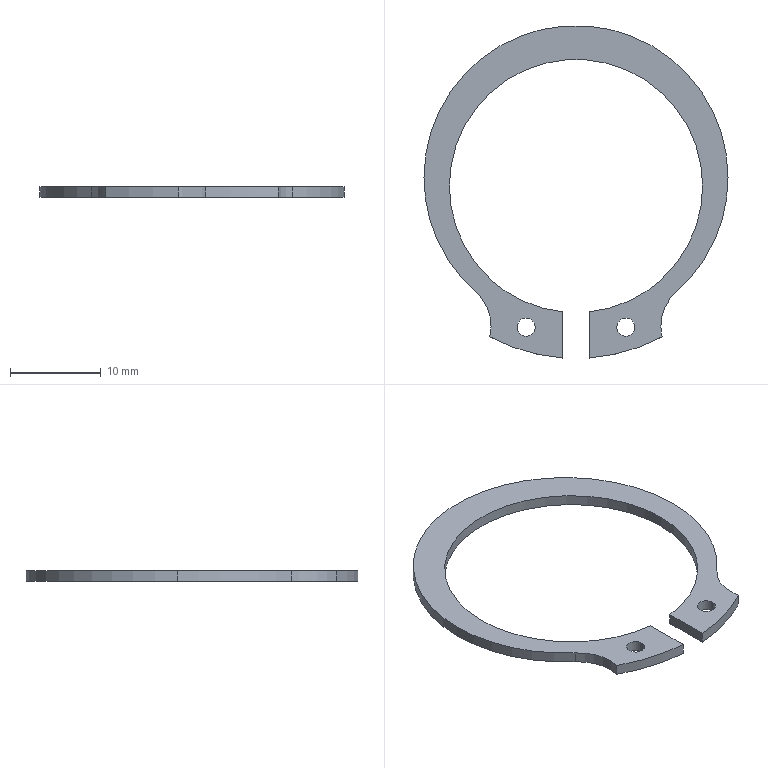Part | SolidWorks | features MBimport 1 | 1 solid | 19 faces | box 33.5 x 36.623 x 1.2 mm | volume 375.357 mm3 | cylinder 15 | plane 4 | commonest cylinder face diameters 2 x4 10 x3 27.9 x3 33.5 x3 39.86 x2
STEP:
#1=CARTESIAN_POINT('',(4.5,-16.486,0.6));
#2=VERTEX_POINT('',#1);
#3=CARTESIAN_POINT('',(6.5,-16.486,0.6));
#4=VERTEX_POINT('',#3);
#5=CARTESIAN_POINT('',(5.5,-16.486,0.6));
#6=DIRECTION('',(0.,0.,1.));
#7=DIRECTION('',(-1.,0.,0.));
#8=AXIS2_PLACEMENT_3D('',#5,#6,#7);
#9=CIRCLE('',#8,1.);
#10=EDGE_CURVE('',#2,#4,#9,.T.);
#11=ORIENTED_EDGE('',*,*,#10,.T.);
#12=CARTESIAN_POINT('',(6.5,-16.486,-0.6));
#13=VERTEX_POINT('',#12);
#14=CARTESIAN_POINT('',(6.5,-16.486,0.6));
#15=DIRECTION('',(0.,0.,-1.));
#16=VECTOR('',#15,1000.);
#17=LINE('',#14,#16);
#18=EDGE_CURVE('',#4,#13,#17,.T.);
#19=ORIENTED_EDGE('',*,*,#18,.T.);
#20=CARTESIAN_POINT('',(4.5,-16.486,-0.6));
#21=VERTEX_POINT('',#20);
#22=CARTESIAN_POINT('',(5.5,-16.486,-0.6));
#23=DIRECTION('',(0.,0.,1.));
#24=DIRECTION('',(-1.,0.,0.));
#25=AXIS2_PLACEMENT_3D('',#22,#23,#24);
#26=CIRCLE('',#25,1.);
#27=EDGE_CURVE('',#21,#13,#26,.T.);
#28=ORIENTED_EDGE('',*,*,#27,.F.);
#29=CARTESIAN_POINT('',(4.5,-16.486,0.6));
#30=DIRECTION('',(0.,0.,-1.));
#31=VECTOR('',#30,1000.);
#32=LINE('',#29,#31);
#33=EDGE_CURVE('',#2,#21,#32,.T.);
#34=ORIENTED_EDGE('',*,*,#33,.F.);
#35=EDGE_LOOP('',(#11,#19,#28,#34));
#36=FACE_OUTER_BOUND('',#35,.T.);
#37=CARTESIAN_POINT('',(5.5,-16.486,0.6));
#38=DIRECTION('',(0.,0.,-1.));
#39=DIRECTION('',(-1.,0.,0.));
#40=AXIS2_PLACEMENT_3D('',#37,#38,#39);
#41=CYLINDRICAL_SURFACE('',#40,1.);
#42=ADVANCED_FACE('',(#36),#41,.F.);
#43=CARTESIAN_POINT('',(-6.5,-16.486,0.6));
#44=VERTEX_POINT('',#43);
#45=CARTESIAN_POINT('',(-4.5,-16.486,0.6));
#46=VERTEX_POINT('',#45);
#47=CARTESIAN_POINT('',(-5.5,-16.486,0.6));
#48=DIRECTION('',(0.,0.,1.));
#49=DIRECTION('',(1.,0.,0.));
#50=AXIS2_PLACEMENT_3D('',#47,#48,#49);
#51=CIRCLE('',#50,1.);
#52=EDGE_CURVE('',#44,#46,#51,.T.);
#53=ORIENTED_EDGE('',*,*,#52,.T.);
#54=CARTESIAN_POINT('',(-4.5,-16.486,-0.6));
#55=VERTEX_POINT('',#54);
#56=CARTESIAN_POINT('',(-4.5,-16.486,0.6));
#57=DIRECTION('',(0.,0.,-1.));
#58=VECTOR('',#57,1000.);
#59=LINE('',#56,#58);
#60=EDGE_CURVE('',#46,#55,#59,.T.);
#61=ORIENTED_EDGE('',*,*,#60,.T.);
#62=CARTESIAN_POINT('',(-6.5,-16.486,-0.6));
#63=VERTEX_POINT('',#62);
#64=CARTESIAN_POINT('',(-5.5,-16.486,-0.6));
#65=DIRECTION('',(0.,0.,1.));
#66=DIRECTION('',(1.,0.,0.));
#67=AXIS2_PLACEMENT_3D('',#64,#65,#66);
#68=CIRCLE('',#67,1.);
#69=EDGE_CURVE('',#63,#55,#68,.T.);
#70=ORIENTED_EDGE('',*,*,#69,.F.);
#71=CARTESIAN_POINT('',(-6.5,-16.486,0.6));
#72=DIRECTION('',(0.,0.,-1.));
#73=VECTOR('',#72,1000.);
#74=LINE('',#71,#73);
#75=EDGE_CURVE('',#44,#63,#74,.T.);
#76=ORIENTED_EDGE('',*,*,#75,.F.);
#77=EDGE_LOOP('',(#53,#61,#70,#76));
#78=FACE_OUTER_BOUND('',#77,.T.);
#79=CARTESIAN_POINT('',(-5.5,-16.486,0.6));
#80=DIRECTION('',(0.,0.,-1.));
#81=DIRECTION('',(-1.,0.,0.));
#82=AXIS2_PLACEMENT_3D('',#79,#80,#81);
#83=CYLINDRICAL_SURFACE('',#82,1.);
#84=ADVANCED_FACE('',(#78),#83,.F.);
#85=CARTESIAN_POINT('',(16.75,0.,0.6));
#86=VERTEX_POINT('',#85);
#87=CARTESIAN_POINT('',(-16.75,0.,0.6));
#88=VERTEX_POINT('',#87);
#89=CARTESIAN_POINT('',(0.,0.,0.6));
#90=DIRECTION('',(0.,0.,1.));
#91=DIRECTION('',(1.,0.,0.));
#92=AXIS2_PLACEMENT_3D('',#89,#90,#91);
#93=CIRCLE('',#92,16.75);
#94=EDGE_CURVE('',#86,#88,#93,.T.);
#95=ORIENTED_EDGE('',*,*,#94,.F.);
#96=CARTESIAN_POINT('',(16.75,0.,-0.6));
#97=VERTEX_POINT('',#96);
#98=CARTESIAN_POINT('',(16.75,0.,0.6));
#99=DIRECTION('',(0.,0.,-1.));
#100=VECTOR('',#99,1000.);
#101=LINE('',#98,#100);
#102=EDGE_CURVE('',#86,#97,#101,.T.);
#103=ORIENTED_EDGE('',*,*,#102,.T.);
#104=CARTESIAN_POINT('',(-16.75,0.,-0.6));
#105=VERTEX_POINT('',#104);
#106=CARTESIAN_POINT('',(0.,0.,-0.6));
#107=DIRECTION('',(0.,0.,1.));
#108=DIRECTION('',(1.,0.,0.));
#109=AXIS2_PLACEMENT_3D('',#106,#107,#108);
#110=CIRCLE('',#109,16.75);
#111=EDGE_CURVE('',#97,#105,#110,.T.);
#112=ORIENTED_EDGE('',*,*,#111,.T.);
#113=CARTESIAN_POINT('',(-16.75,0.,0.6));
#114=DIRECTION('',(0.,0.,-1.));
#115=VECTOR('',#114,1000.);
#116=LINE('',#113,#115);
#117=EDGE_CURVE('',#88,#105,#116,.T.);
#118=ORIENTED_EDGE('',*,*,#117,.F.);
#119=EDGE_LOOP('',(#95,#103,#112,#118));
#120=FACE_OUTER_BOUND('',#119,.T.);
#121=CARTESIAN_POINT('',(0.,0.,0.6));
#122=DIRECTION('',(0.,0.,-1.));
#123=DIRECTION('',(-1.,0.,0.));
#124=AXIS2_PLACEMENT_3D('',#121,#122,#123);
#125=CYLINDRICAL_SURFACE('',#124,16.75);
#126=ADVANCED_FACE('',(#120),#125,.T.);
#127=CARTESIAN_POINT('',(-11.057,-12.582,0.6));
#128=VERTEX_POINT('',#127);
#129=CARTESIAN_POINT('',(0.,0.,0.6));
#130=DIRECTION('',(0.,0.,1.));
#131=DIRECTION('',(1.,0.,0.));
#132=AXIS2_PLACEMENT_3D('',#129,#130,#131);
#133=CIRCLE('',#132,16.75);
#134=EDGE_CURVE('',#88,#128,#133,.T.);
#135=ORIENTED_EDGE('',*,*,#134,.F.);
#136=ORIENTED_EDGE('',*,*,#117,.T.);
#137=CARTESIAN_POINT('',(-11.057,-12.582,-0.6));
#138=VERTEX_POINT('',#137);
#139=CARTESIAN_POINT('',(0.,0.,-0.6));
#140=DIRECTION('',(0.,0.,1.));
#141=DIRECTION('',(1.,0.,0.));
#142=AXIS2_PLACEMENT_3D('',#139,#140,#141);
#143=CIRCLE('',#142,16.75);
#144=EDGE_CURVE('',#105,#138,#143,.T.);
#145=ORIENTED_EDGE('',*,*,#144,.T.);
#146=CARTESIAN_POINT('',(-11.057,-12.582,0.6));
#147=DIRECTION('',(0.,0.,-1.));
#148=VECTOR('',#147,1000.);
#149=LINE('',#146,#148);
#150=EDGE_CURVE('',#128,#138,#149,.T.);
#151=ORIENTED_EDGE('',*,*,#150,.F.);
#152=EDGE_LOOP('',(#135,#136,#145,#151));
#153=FACE_OUTER_BOUND('',#152,.T.);
#154=CARTESIAN_POINT('',(0.,0.,0.6));
#155=DIRECTION('',(0.,0.,-1.));
#156=DIRECTION('',(-1.,0.,0.));
#157=AXIS2_PLACEMENT_3D('',#154,#155,#156);
#158=CYLINDRICAL_SURFACE('',#157,16.75);
#159=ADVANCED_FACE('',(#153),#158,.T.);
#160=CARTESIAN_POINT('',(9.358,-16.337,0.6));
#161=VERTEX_POINT('',#160);
#162=CARTESIAN_POINT('',(11.057,-12.582,0.6));
#163=VERTEX_POINT('',#162);
#164=CARTESIAN_POINT('',(14.358,-16.337,0.6));
#165=DIRECTION('',(0.,0.,-1.));
#166=DIRECTION('',(-1.,0.,0.));
#167=AXIS2_PLACEMENT_3D('',#164,#165,#166);
#168=CIRCLE('',#167,5.);
#169=EDGE_CURVE('',#161,#163,#168,.T.);
#170=ORIENTED_EDGE('',*,*,#169,.F.);
#171=CARTESIAN_POINT('',(9.358,-16.337,-0.6));
#172=VERTEX_POINT('',#171);
#173=CARTESIAN_POINT('',(9.358,-16.337,0.6));
#174=DIRECTION('',(0.,0.,-1.));
#175=VECTOR('',#174,1000.);
#176=LINE('',#173,#175);
#177=EDGE_CURVE('',#161,#172,#176,.T.);
#178=ORIENTED_EDGE('',*,*,#177,.T.);
#179=CARTESIAN_POINT('',(11.057,-12.582,-0.6));
#180=VERTEX_POINT('',#179);
#181=CARTESIAN_POINT('',(14.358,-16.337,-0.6));
#182=DIRECTION('',(0.,0.,-1.));
#183=DIRECTION('',(-1.,0.,0.));
#184=AXIS2_PLACEMENT_3D('',#181,#182,#183);
#185=CIRCLE('',#184,5.);
#186=EDGE_CURVE('',#172,#180,#185,.T.);
#187=ORIENTED_EDGE('',*,*,#186,.T.);
#188=CARTESIAN_POINT('',(11.057,-12.582,0.6));
#189=DIRECTION('',(0.,0.,-1.));
#190=VECTOR('',#189,1000.);
#191=LINE('',#188,#190);
#192=EDGE_CURVE('',#163,#180,#191,.T.);
#193=ORIENTED_EDGE('',*,*,#192,.F.);
#194=EDGE_LOOP('',(#170,#178,#187,#193));
#195=FACE_OUTER_BOUND('',#194,.T.);
#196=CARTESIAN_POINT('',(14.358,-16.337,0.6));
#197=DIRECTION('',(0.,0.,-1.));
#198=DIRECTION('',(-1.,0.,0.));
#199=AXIS2_PLACEMENT_3D('',#196,#197,#198);
#200=CYLINDRICAL_SURFACE('',#199,5.);
#201=ADVANCED_FACE('',(#195),#200,.F.);
#202=CARTESIAN_POINT('',(13.95,-0.93,0.6));
#203=VERTEX_POINT('',#202);
#204=CARTESIAN_POINT('',(1.5,-14.799,0.6));
#205=VERTEX_POINT('',#204);
#206=CARTESIAN_POINT('',(0.,-0.93,0.6));
#207=DIRECTION('',(0.,0.,-1.));
#208=DIRECTION('',(1.,0.,0.));
#209=AXIS2_PLACEMENT_3D('',#206,#207,#208);
#210=CIRCLE('',#209,13.95);
#211=EDGE_CURVE('',#203,#205,#210,.T.);
#212=ORIENTED_EDGE('',*,*,#211,.F.);
#213=CARTESIAN_POINT('',(13.95,-0.93,-0.6));
#214=VERTEX_POINT('',#213);
#215=CARTESIAN_POINT('',(13.95,-0.93,0.6));
#216=DIRECTION('',(0.,0.,-1.));
#217=VECTOR('',#216,1000.);
#218=LINE('',#215,#217);
#219=EDGE_CURVE('',#203,#214,#218,.T.);
#220=ORIENTED_EDGE('',*,*,#219,.T.);
#221=CARTESIAN_POINT('',(1.5,-14.799,-0.6));
#222=VERTEX_POINT('',#221);
#223=CARTESIAN_POINT('',(0.,-0.93,-0.6));
#224=DIRECTION('',(0.,0.,-1.));
#225=DIRECTION('',(1.,0.,0.));
#226=AXIS2_PLACEMENT_3D('',#223,#224,#225);
#227=CIRCLE('',#226,13.95);
#228=EDGE_CURVE('',#214,#222,#227,.T.);
#229=ORIENTED_EDGE('',*,*,#228,.T.);
#230=CARTESIAN_POINT('',(1.5,-14.799,0.6));
#231=DIRECTION('',(0.,0.,-1.));
#232=VECTOR('',#231,1000.);
#233=LINE('',#230,#232);
#234=EDGE_CURVE('',#205,#222,#233,.T.);
#235=ORIENTED_EDGE('',*,*,#234,.F.);
#236=EDGE_LOOP('',(#212,#220,#229,#235));
#237=FACE_OUTER_BOUND('',#236,.T.);
#238=CARTESIAN_POINT('',(0.,-0.93,0.6));
#239=DIRECTION('',(0.,0.,-1.));
#240=DIRECTION('',(-1.,0.,0.));
#241=AXIS2_PLACEMENT_3D('',#238,#239,#240);
#242=CYLINDRICAL_SURFACE('',#241,13.95);
#243=ADVANCED_FACE('',(#237),#242,.F.);
#244=ORIENTED_EDGE('',*,*,#219,.F.);
#245=CARTESIAN_POINT('',(-13.95,-0.93,0.6));
#246=VERTEX_POINT('',#245);
#247=CARTESIAN_POINT('',(0.,-0.93,0.6));
#248=DIRECTION('',(0.,0.,-1.));
#249=DIRECTION('',(1.,0.,0.));
#250=AXIS2_PLACEMENT_3D('',#247,#248,#249);
#251=CIRCLE('',#250,13.95);
#252=EDGE_CURVE('',#246,#203,#251,.T.);
#253=ORIENTED_EDGE('',*,*,#252,.F.);
#254=CARTESIAN_POINT('',(-13.95,-0.93,-0.6));
#255=VERTEX_POINT('',#254);
#256=CARTESIAN_POINT('',(-13.95,-0.93,0.6));
#257=DIRECTION('',(0.,0.,-1.));
#258=VECTOR('',#257,1000.);
#259=LINE('',#256,#258);
#260=EDGE_CURVE('',#246,#255,#259,.T.);
#261=ORIENTED_EDGE('',*,*,#260,.T.);
#262=CARTESIAN_POINT('',(0.,-0.93,-0.6));
#263=DIRECTION('',(0.,0.,-1.));
#264=DIRECTION('',(1.,0.,0.));
#265=AXIS2_PLACEMENT_3D('',#262,#263,#264);
#266=CIRCLE('',#265,13.95);
#267=EDGE_CURVE('',#255,#214,#266,.T.);
#268=ORIENTED_EDGE('',*,*,#267,.T.);
#269=EDGE_LOOP('',(#244,#253,#261,#268));
#270=FACE_OUTER_BOUND('',#269,.T.);
#271=CARTESIAN_POINT('',(0.,-0.93,0.6));
#272=DIRECTION('',(0.,0.,-1.));
#273=DIRECTION('',(-1.,0.,0.));
#274=AXIS2_PLACEMENT_3D('',#271,#272,#273);
#275=CYLINDRICAL_SURFACE('',#274,13.95);
#276=ADVANCED_FACE('',(#270),#275,.F.);
#277=CARTESIAN_POINT('',(-1.5,-14.799,0.6));
#278=VERTEX_POINT('',#277);
#279=CARTESIAN_POINT('',(0.,-0.93,0.6));
#280=DIRECTION('',(0.,0.,-1.));
#281=DIRECTION('',(1.,0.,0.));
#282=AXIS2_PLACEMENT_3D('',#279,#280,#281);
#283=CIRCLE('',#282,13.95);
#284=EDGE_CURVE('',#278,#246,#283,.T.);
#285=ORIENTED_EDGE('',*,*,#284,.T.);
#286=ORIENTED_EDGE('',*,*,#252,.T.);
#287=ORIENTED_EDGE('',*,*,#211,.T.);
#288=CARTESIAN_POINT('',(1.5,-19.873,0.6));
#289=VERTEX_POINT('',#288);
#290=CARTESIAN_POINT('',(1.5,-14.799,0.6));
#291=DIRECTION('',(0.,-1.,0.));
#292=VECTOR('',#291,1000.);
#293=LINE('',#290,#292);
#294=EDGE_CURVE('',#205,#289,#293,.T.);
#295=ORIENTED_EDGE('',*,*,#294,.T.);
#296=CARTESIAN_POINT('',(9.5,-17.52,0.6));
#297=VERTEX_POINT('',#296);
#298=CARTESIAN_POINT('',(0.,0.,0.6));
#299=DIRECTION('',(0.,0.,1.));
#300=DIRECTION('',(1.,0.,0.));
#301=AXIS2_PLACEMENT_3D('',#298,#299,#300);
#302=CIRCLE('',#301,19.93);
#303=EDGE_CURVE('',#289,#297,#302,.T.);
#304=ORIENTED_EDGE('',*,*,#303,.T.);
#305=CARTESIAN_POINT('',(14.358,-16.337,0.6));
#306=DIRECTION('',(0.,0.,-1.));
#307=DIRECTION('',(-1.,0.,0.));
#308=AXIS2_PLACEMENT_3D('',#305,#306,#307);
#309=CIRCLE('',#308,5.);
#310=EDGE_CURVE('',#297,#161,#309,.T.);
#311=ORIENTED_EDGE('',*,*,#310,.T.);
#312=ORIENTED_EDGE('',*,*,#169,.T.);
#313=CARTESIAN_POINT('',(0.,0.,0.6));
#314=DIRECTION('',(0.,0.,1.));
#315=DIRECTION('',(1.,0.,0.));
#316=AXIS2_PLACEMENT_3D('',#313,#314,#315);
#317=CIRCLE('',#316,16.75);
#318=EDGE_CURVE('',#163,#86,#317,.T.);
#319=ORIENTED_EDGE('',*,*,#318,.T.);
#320=ORIENTED_EDGE('',*,*,#94,.T.);
#321=ORIENTED_EDGE('',*,*,#134,.T.);
#322=CARTESIAN_POINT('',(-9.5,-17.52,0.6));
#323=VERTEX_POINT('',#322);
#324=CARTESIAN_POINT('',(-14.358,-16.337,0.6));
#325=DIRECTION('',(0.,0.,-1.));
#326=DIRECTION('',(1.,0.,0.));
#327=AXIS2_PLACEMENT_3D('',#324,#325,#326);
#328=CIRCLE('',#327,5.);
#329=EDGE_CURVE('',#128,#323,#328,.T.);
#330=ORIENTED_EDGE('',*,*,#329,.T.);
#331=CARTESIAN_POINT('',(-1.5,-19.873,0.6));
#332=VERTEX_POINT('',#331);
#333=CARTESIAN_POINT('',(0.,0.,0.6));
#334=DIRECTION('',(0.,0.,1.));
#335=DIRECTION('',(-1.,0.,0.));
#336=AXIS2_PLACEMENT_3D('',#333,#334,#335);
#337=CIRCLE('',#336,19.93);
#338=EDGE_CURVE('',#323,#332,#337,.T.);
#339=ORIENTED_EDGE('',*,*,#338,.T.);
#340=CARTESIAN_POINT('',(-1.5,-14.799,0.6));
#341=DIRECTION('',(0.,1.,0.));
#342=VECTOR('',#341,1000.);
#343=LINE('',#340,#342);
#344=EDGE_CURVE('',#332,#278,#343,.T.);
#345=ORIENTED_EDGE('',*,*,#344,.T.);
#346=EDGE_LOOP('',(#285,#286,#287,#295,#304,#311,#312,#319,#320,#321,#330,#339,#345));
#347=FACE_OUTER_BOUND('',#346,.T.);
#348=ORIENTED_EDGE('',*,*,#52,.F.);
#349=CARTESIAN_POINT('',(-5.5,-16.486,0.6));
#350=DIRECTION('',(0.,0.,1.));
#351=DIRECTION('',(1.,0.,0.));
#352=AXIS2_PLACEMENT_3D('',#349,#350,#351);
#353=CIRCLE('',#352,1.);
#354=EDGE_CURVE('',#46,#44,#353,.T.);
#355=ORIENTED_EDGE('',*,*,#354,.F.);
#356=EDGE_LOOP('',(#348,#355));
#357=FACE_BOUND('',#356,.T.);
#358=ORIENTED_EDGE('',*,*,#10,.F.);
#359=CARTESIAN_POINT('',(5.5,-16.486,0.6));
#360=DIRECTION('',(0.,0.,1.));
#361=DIRECTION('',(-1.,0.,0.));
#362=AXIS2_PLACEMENT_3D('',#359,#360,#361);
#363=CIRCLE('',#362,1.);
#364=EDGE_CURVE('',#4,#2,#363,.T.);
#365=ORIENTED_EDGE('',*,*,#364,.F.);
#366=EDGE_LOOP('',(#358,#365));
#367=FACE_BOUND('',#366,.T.);
#368=CARTESIAN_POINT('',(0.,-0.93,0.6));
#369=DIRECTION('',(0.,0.,1.));
#370=DIRECTION('',(1.,0.,0.));
#371=AXIS2_PLACEMENT_3D('',#368,#369,#370);
#372=PLANE('',#371);
#373=ADVANCED_FACE('',(#347,#357,#367),#372,.T.);
#374=ORIENTED_EDGE('',*,*,#260,.F.);
#375=ORIENTED_EDGE('',*,*,#284,.F.);
#376=CARTESIAN_POINT('',(-1.5,-14.799,-0.6));
#377=VERTEX_POINT('',#376);
#378=CARTESIAN_POINT('',(-1.5,-14.799,0.6));
#379=DIRECTION('',(0.,0.,-1.));
#380=VECTOR('',#379,1000.);
#381=LINE('',#378,#380);
#382=EDGE_CURVE('',#278,#377,#381,.T.);
#383=ORIENTED_EDGE('',*,*,#382,.T.);
#384=CARTESIAN_POINT('',(0.,-0.93,-0.6));
#385=DIRECTION('',(0.,0.,-1.));
#386=DIRECTION('',(1.,0.,0.));
#387=AXIS2_PLACEMENT_3D('',#384,#385,#386);
#388=CIRCLE('',#387,13.95);
#389=EDGE_CURVE('',#377,#255,#388,.T.);
#390=ORIENTED_EDGE('',*,*,#389,.T.);
#391=EDGE_LOOP('',(#374,#375,#383,#390));
#392=FACE_OUTER_BOUND('',#391,.T.);
#393=CARTESIAN_POINT('',(0.,-0.93,0.6));
#394=DIRECTION('',(0.,0.,-1.));
#395=DIRECTION('',(-1.,0.,0.));
#396=AXIS2_PLACEMENT_3D('',#393,#394,#395);
#397=CYLINDRICAL_SURFACE('',#396,13.95);
#398=ADVANCED_FACE('',(#392),#397,.F.);
#399=ORIENTED_EDGE('',*,*,#234,.T.);
#400=CARTESIAN_POINT('',(1.5,-19.873,-0.6));
#401=VERTEX_POINT('',#400);
#402=CARTESIAN_POINT('',(1.5,-14.799,-0.6));
#403=DIRECTION('',(0.,-1.,0.));
#404=VECTOR('',#403,1000.);
#405=LINE('',#402,#404);
#406=EDGE_CURVE('',#222,#401,#405,.T.);
#407=ORIENTED_EDGE('',*,*,#406,.T.);
#408=CARTESIAN_POINT('',(1.5,-19.873,0.6));
#409=DIRECTION('',(0.,0.,-1.));
#410=VECTOR('',#409,1000.);
#411=LINE('',#408,#410);
#412=EDGE_CURVE('',#289,#401,#411,.T.);
#413=ORIENTED_EDGE('',*,*,#412,.F.);
#414=ORIENTED_EDGE('',*,*,#294,.F.);
#415=EDGE_LOOP('',(#399,#407,#413,#414));
#416=FACE_OUTER_BOUND('',#415,.T.);
#417=CARTESIAN_POINT('',(1.5,-14.799,0.6));
#418=DIRECTION('',(1.,0.,0.));
#419=DIRECTION('',(0.,1.,0.));
#420=AXIS2_PLACEMENT_3D('',#417,#418,#419);
#421=PLANE('',#420);
#422=ADVANCED_FACE('',(#416),#421,.F.);
#423=ORIENTED_EDGE('',*,*,#412,.T.);
#424=CARTESIAN_POINT('',(9.5,-17.52,-0.6));
#425=VERTEX_POINT('',#424);
#426=CARTESIAN_POINT('',(0.,0.,-0.6));
#427=DIRECTION('',(0.,0.,1.));
#428=DIRECTION('',(1.,0.,0.));
#429=AXIS2_PLACEMENT_3D('',#426,#427,#428);
#430=CIRCLE('',#429,19.93);
#431=EDGE_CURVE('',#401,#425,#430,.T.);
#432=ORIENTED_EDGE('',*,*,#431,.T.);
#433=CARTESIAN_POINT('',(9.5,-17.52,0.6));
#434=DIRECTION('',(0.,0.,-1.));
#435=VECTOR('',#434,1000.);
#436=LINE('',#433,#435);
#437=EDGE_CURVE('',#297,#425,#436,.T.);
#438=ORIENTED_EDGE('',*,*,#437,.F.);
#439=ORIENTED_EDGE('',*,*,#303,.F.);
#440=EDGE_LOOP('',(#423,#432,#438,#439));
#441=FACE_OUTER_BOUND('',#440,.T.);
#442=CARTESIAN_POINT('',(0.,0.,0.6));
#443=DIRECTION('',(0.,0.,-1.));
#444=DIRECTION('',(-1.,0.,0.));
#445=AXIS2_PLACEMENT_3D('',#442,#443,#444);
#446=CYLINDRICAL_SURFACE('',#445,19.93);
#447=ADVANCED_FACE('',(#441),#446,.T.);
#448=ORIENTED_EDGE('',*,*,#177,.F.);
#449=ORIENTED_EDGE('',*,*,#310,.F.);
#450=ORIENTED_EDGE('',*,*,#437,.T.);
#451=CARTESIAN_POINT('',(14.358,-16.337,-0.6));
#452=DIRECTION('',(0.,0.,-1.));
#453=DIRECTION('',(-1.,0.,0.));
#454=AXIS2_PLACEMENT_3D('',#451,#452,#453);
#455=CIRCLE('',#454,5.);
#456=EDGE_CURVE('',#425,#172,#455,.T.);
#457=ORIENTED_EDGE('',*,*,#456,.T.);
#458=EDGE_LOOP('',(#448,#449,#450,#457));
#459=FACE_OUTER_BOUND('',#458,.T.);
#460=CARTESIAN_POINT('',(14.358,-16.337,0.6));
#461=DIRECTION('',(0.,0.,-1.));
#462=DIRECTION('',(-1.,0.,0.));
#463=AXIS2_PLACEMENT_3D('',#460,#461,#462);
#464=CYLINDRICAL_SURFACE('',#463,5.);
#465=ADVANCED_FACE('',(#459),#464,.F.);
#466=ORIENTED_EDGE('',*,*,#102,.F.);
#467=ORIENTED_EDGE('',*,*,#318,.F.);
#468=ORIENTED_EDGE('',*,*,#192,.T.);
#469=CARTESIAN_POINT('',(0.,0.,-0.6));
#470=DIRECTION('',(0.,0.,1.));
#471=DIRECTION('',(1.,0.,0.));
#472=AXIS2_PLACEMENT_3D('',#469,#470,#471);
#473=CIRCLE('',#472,16.75);
#474=EDGE_CURVE('',#180,#97,#473,.T.);
#475=ORIENTED_EDGE('',*,*,#474,.T.);
#476=EDGE_LOOP('',(#466,#467,#468,#475));
#477=FACE_OUTER_BOUND('',#476,.T.);
#478=CARTESIAN_POINT('',(0.,0.,0.6));
#479=DIRECTION('',(0.,0.,-1.));
#480=DIRECTION('',(-1.,0.,0.));
#481=AXIS2_PLACEMENT_3D('',#478,#479,#480);
#482=CYLINDRICAL_SURFACE('',#481,16.75);
#483=ADVANCED_FACE('',(#477),#482,.T.);
#484=ORIENTED_EDGE('',*,*,#150,.T.);
#485=CARTESIAN_POINT('',(-9.5,-17.52,-0.6));
#486=VERTEX_POINT('',#485);
#487=CARTESIAN_POINT('',(-14.358,-16.337,-0.6));
#488=DIRECTION('',(0.,0.,-1.));
#489=DIRECTION('',(1.,0.,0.));
#490=AXIS2_PLACEMENT_3D('',#487,#488,#489);
#491=CIRCLE('',#490,5.);
#492=EDGE_CURVE('',#138,#486,#491,.T.);
#493=ORIENTED_EDGE('',*,*,#492,.T.);
#494=CARTESIAN_POINT('',(-9.5,-17.52,0.6));
#495=DIRECTION('',(0.,0.,-1.));
#496=VECTOR('',#495,1000.);
#497=LINE('',#494,#496);
#498=EDGE_CURVE('',#323,#486,#497,.T.);
#499=ORIENTED_EDGE('',*,*,#498,.F.);
#500=ORIENTED_EDGE('',*,*,#329,.F.);
#501=EDGE_LOOP('',(#484,#493,#499,#500));
#502=FACE_OUTER_BOUND('',#501,.T.);
#503=CARTESIAN_POINT('',(-14.358,-16.337,0.6));
#504=DIRECTION('',(0.,0.,-1.));
#505=DIRECTION('',(-1.,0.,0.));
#506=AXIS2_PLACEMENT_3D('',#503,#504,#505);
#507=CYLINDRICAL_SURFACE('',#506,5.);
#508=ADVANCED_FACE('',(#502),#507,.F.);
#509=ORIENTED_EDGE('',*,*,#498,.T.);
#510=CARTESIAN_POINT('',(-1.5,-19.873,-0.6));
#511=VERTEX_POINT('',#510);
#512=CARTESIAN_POINT('',(0.,0.,-0.6));
#513=DIRECTION('',(0.,0.,1.));
#514=DIRECTION('',(-1.,0.,0.));
#515=AXIS2_PLACEMENT_3D('',#512,#513,#514);
#516=CIRCLE('',#515,19.93);
#517=EDGE_CURVE('',#486,#511,#516,.T.);
#518=ORIENTED_EDGE('',*,*,#517,.T.);
#519=CARTESIAN_POINT('',(-1.5,-19.873,0.6));
#520=DIRECTION('',(0.,0.,-1.));
#521=VECTOR('',#520,1000.);
#522=LINE('',#519,#521);
#523=EDGE_CURVE('',#332,#511,#522,.T.);
#524=ORIENTED_EDGE('',*,*,#523,.F.);
#525=ORIENTED_EDGE('',*,*,#338,.F.);
#526=EDGE_LOOP('',(#509,#518,#524,#525));
#527=FACE_OUTER_BOUND('',#526,.T.);
#528=CARTESIAN_POINT('',(0.,0.,0.6));
#529=DIRECTION('',(0.,0.,-1.));
#530=DIRECTION('',(-1.,0.,0.));
#531=AXIS2_PLACEMENT_3D('',#528,#529,#530);
#532=CYLINDRICAL_SURFACE('',#531,19.93);
#533=ADVANCED_FACE('',(#527),#532,.T.);
#534=ORIENTED_EDGE('',*,*,#523,.T.);
#535=CARTESIAN_POINT('',(-1.5,-14.799,-0.6));
#536=DIRECTION('',(0.,1.,0.));
#537=VECTOR('',#536,1000.);
#538=LINE('',#535,#537);
#539=EDGE_CURVE('',#511,#377,#538,.T.);
#540=ORIENTED_EDGE('',*,*,#539,.T.);
#541=ORIENTED_EDGE('',*,*,#382,.F.);
#542=ORIENTED_EDGE('',*,*,#344,.F.);
#543=EDGE_LOOP('',(#534,#540,#541,#542));
#544=FACE_OUTER_BOUND('',#543,.T.);
#545=CARTESIAN_POINT('',(-1.5,-14.799,0.6));
#546=DIRECTION('',(-1.,0.,0.));
#547=DIRECTION('',(0.,1.,0.));
#548=AXIS2_PLACEMENT_3D('',#545,#546,#547);
#549=PLANE('',#548);
#550=ADVANCED_FACE('',(#544),#549,.F.);
#551=ORIENTED_EDGE('',*,*,#60,.F.);
#552=ORIENTED_EDGE('',*,*,#354,.T.);
#553=ORIENTED_EDGE('',*,*,#75,.T.);
#554=CARTESIAN_POINT('',(-5.5,-16.486,-0.6));
#555=DIRECTION('',(0.,0.,1.));
#556=DIRECTION('',(1.,0.,0.));
#557=AXIS2_PLACEMENT_3D('',#554,#555,#556);
#558=CIRCLE('',#557,1.);
#559=EDGE_CURVE('',#55,#63,#558,.T.);
#560=ORIENTED_EDGE('',*,*,#559,.F.);
#561=EDGE_LOOP('',(#551,#552,#553,#560));
#562=FACE_OUTER_BOUND('',#561,.T.);
#563=CARTESIAN_POINT('',(-5.5,-16.486,0.6));
#564=DIRECTION('',(0.,0.,-1.));
#565=DIRECTION('',(-1.,0.,0.));
#566=AXIS2_PLACEMENT_3D('',#563,#564,#565);
#567=CYLINDRICAL_SURFACE('',#566,1.);
#568=ADVANCED_FACE('',(#562),#567,.F.);
#569=ORIENTED_EDGE('',*,*,#18,.F.);
#570=ORIENTED_EDGE('',*,*,#364,.T.);
#571=ORIENTED_EDGE('',*,*,#33,.T.);
#572=CARTESIAN_POINT('',(5.5,-16.486,-0.6));
#573=DIRECTION('',(0.,0.,1.));
#574=DIRECTION('',(-1.,0.,0.));
#575=AXIS2_PLACEMENT_3D('',#572,#573,#574);
#576=CIRCLE('',#575,1.);
#577=EDGE_CURVE('',#13,#21,#576,.T.);
#578=ORIENTED_EDGE('',*,*,#577,.F.);
#579=EDGE_LOOP('',(#569,#570,#571,#578));
#580=FACE_OUTER_BOUND('',#579,.T.);
#581=CARTESIAN_POINT('',(5.5,-16.486,0.6));
#582=DIRECTION('',(0.,0.,-1.));
#583=DIRECTION('',(-1.,0.,0.));
#584=AXIS2_PLACEMENT_3D('',#581,#582,#583);
#585=CYLINDRICAL_SURFACE('',#584,1.);
#586=ADVANCED_FACE('',(#580),#585,.F.);
#587=ORIENTED_EDGE('',*,*,#389,.F.);
#588=ORIENTED_EDGE('',*,*,#539,.F.);
#589=ORIENTED_EDGE('',*,*,#517,.F.);
#590=ORIENTED_EDGE('',*,*,#492,.F.);
#591=ORIENTED_EDGE('',*,*,#144,.F.);
#592=ORIENTED_EDGE('',*,*,#111,.F.);
#593=ORIENTED_EDGE('',*,*,#474,.F.);
#594=ORIENTED_EDGE('',*,*,#186,.F.);
#595=ORIENTED_EDGE('',*,*,#456,.F.);
#596=ORIENTED_EDGE('',*,*,#431,.F.);
#597=ORIENTED_EDGE('',*,*,#406,.F.);
#598=ORIENTED_EDGE('',*,*,#228,.F.);
#599=ORIENTED_EDGE('',*,*,#267,.F.);
#600=EDGE_LOOP('',(#587,#588,#589,#590,#591,#592,#593,#594,#595,#596,#597,#598,#599));
#601=FACE_OUTER_BOUND('',#600,.T.);
#602=ORIENTED_EDGE('',*,*,#27,.T.);
#603=ORIENTED_EDGE('',*,*,#577,.T.);
#604=EDGE_LOOP('',(#602,#603));
#605=FACE_BOUND('',#604,.T.);
#606=ORIENTED_EDGE('',*,*,#69,.T.);
#607=ORIENTED_EDGE('',*,*,#559,.T.);
#608=EDGE_LOOP('',(#606,#607));
#609=FACE_BOUND('',#608,.T.);
#610=CARTESIAN_POINT('',(0.,-0.93,-0.6));
#611=DIRECTION('',(0.,0.,1.));
#612=DIRECTION('',(1.,0.,0.));
#613=AXIS2_PLACEMENT_3D('',#610,#611,#612);
#614=PLANE('',#613);
#615=ADVANCED_FACE('',(#601,#605,#609),#614,.F.);
#616=CLOSED_SHELL('',(#42,#84,#126,#159,#201,#243,#276,#373,#398,#422,#447,#465,#483,#508,#533,#550,#568,#586,#615));
#617=MANIFOLD_SOLID_BREP('',#616);
#618=CARTESIAN_POINT('',(0.,0.,0.));
#619=DIRECTION('',(0.,0.,1.));
#620=DIRECTION('',(1.,0.,0.));
#621=AXIS2_PLACEMENT_3D('',#618,#619,#620);
#622=(LENGTH_UNIT()NAMED_UNIT(*)SI_UNIT(.MILLI.,.METRE.));
#623=UNCERTAINTY_MEASURE_WITH_UNIT(LENGTH_MEASURE(0.00001),#622,'','');
#624=(NAMED_UNIT(*)PLANE_ANGLE_UNIT()SI_UNIT($,.RADIAN.));
#625=(NAMED_UNIT(*)SI_UNIT($,.STERADIAN.)SOLID_ANGLE_UNIT());
#626=(GEOMETRIC_REPRESENTATION_CONTEXT(3)GLOBAL_UNCERTAINTY_ASSIGNED_CONTEXT((#623))GLOBAL_UNIT_ASSIGNED_CONTEXT((#622,#624,#625))REPRESENTATION_CONTEXT('',''));
#627=ADVANCED_BREP_SHAPE_REPRESENTATION('',(#617,#621),#626);